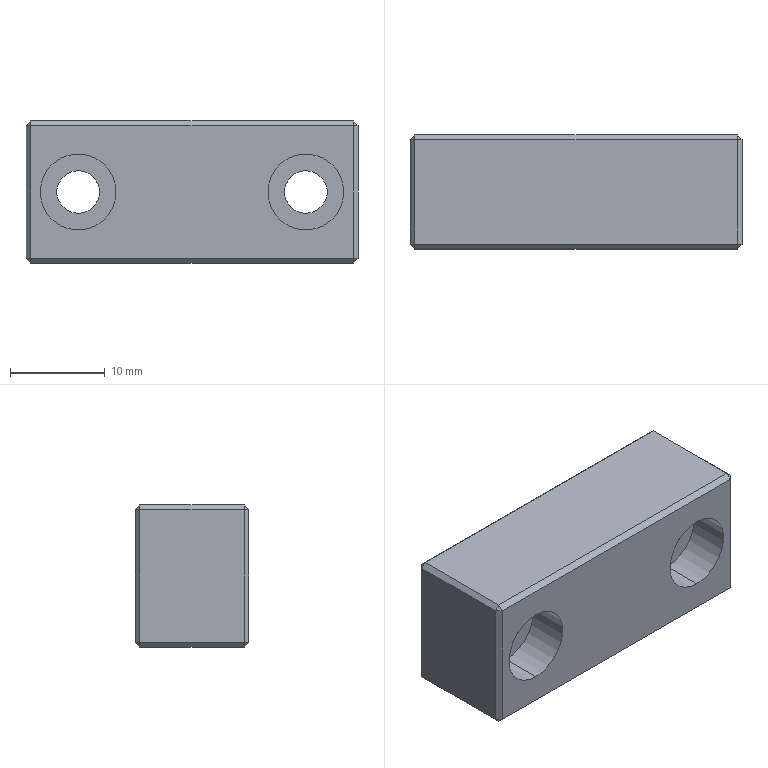Part | STEP file | ND25021-01-JDKM-31-TL | 1 solid | 36 faces | box 35 x 12 x 15 mm | volume 5586 mm3 | plane 28 | cylinder 8 | commonest cylinder face diameters 4.5 x4 8 x4